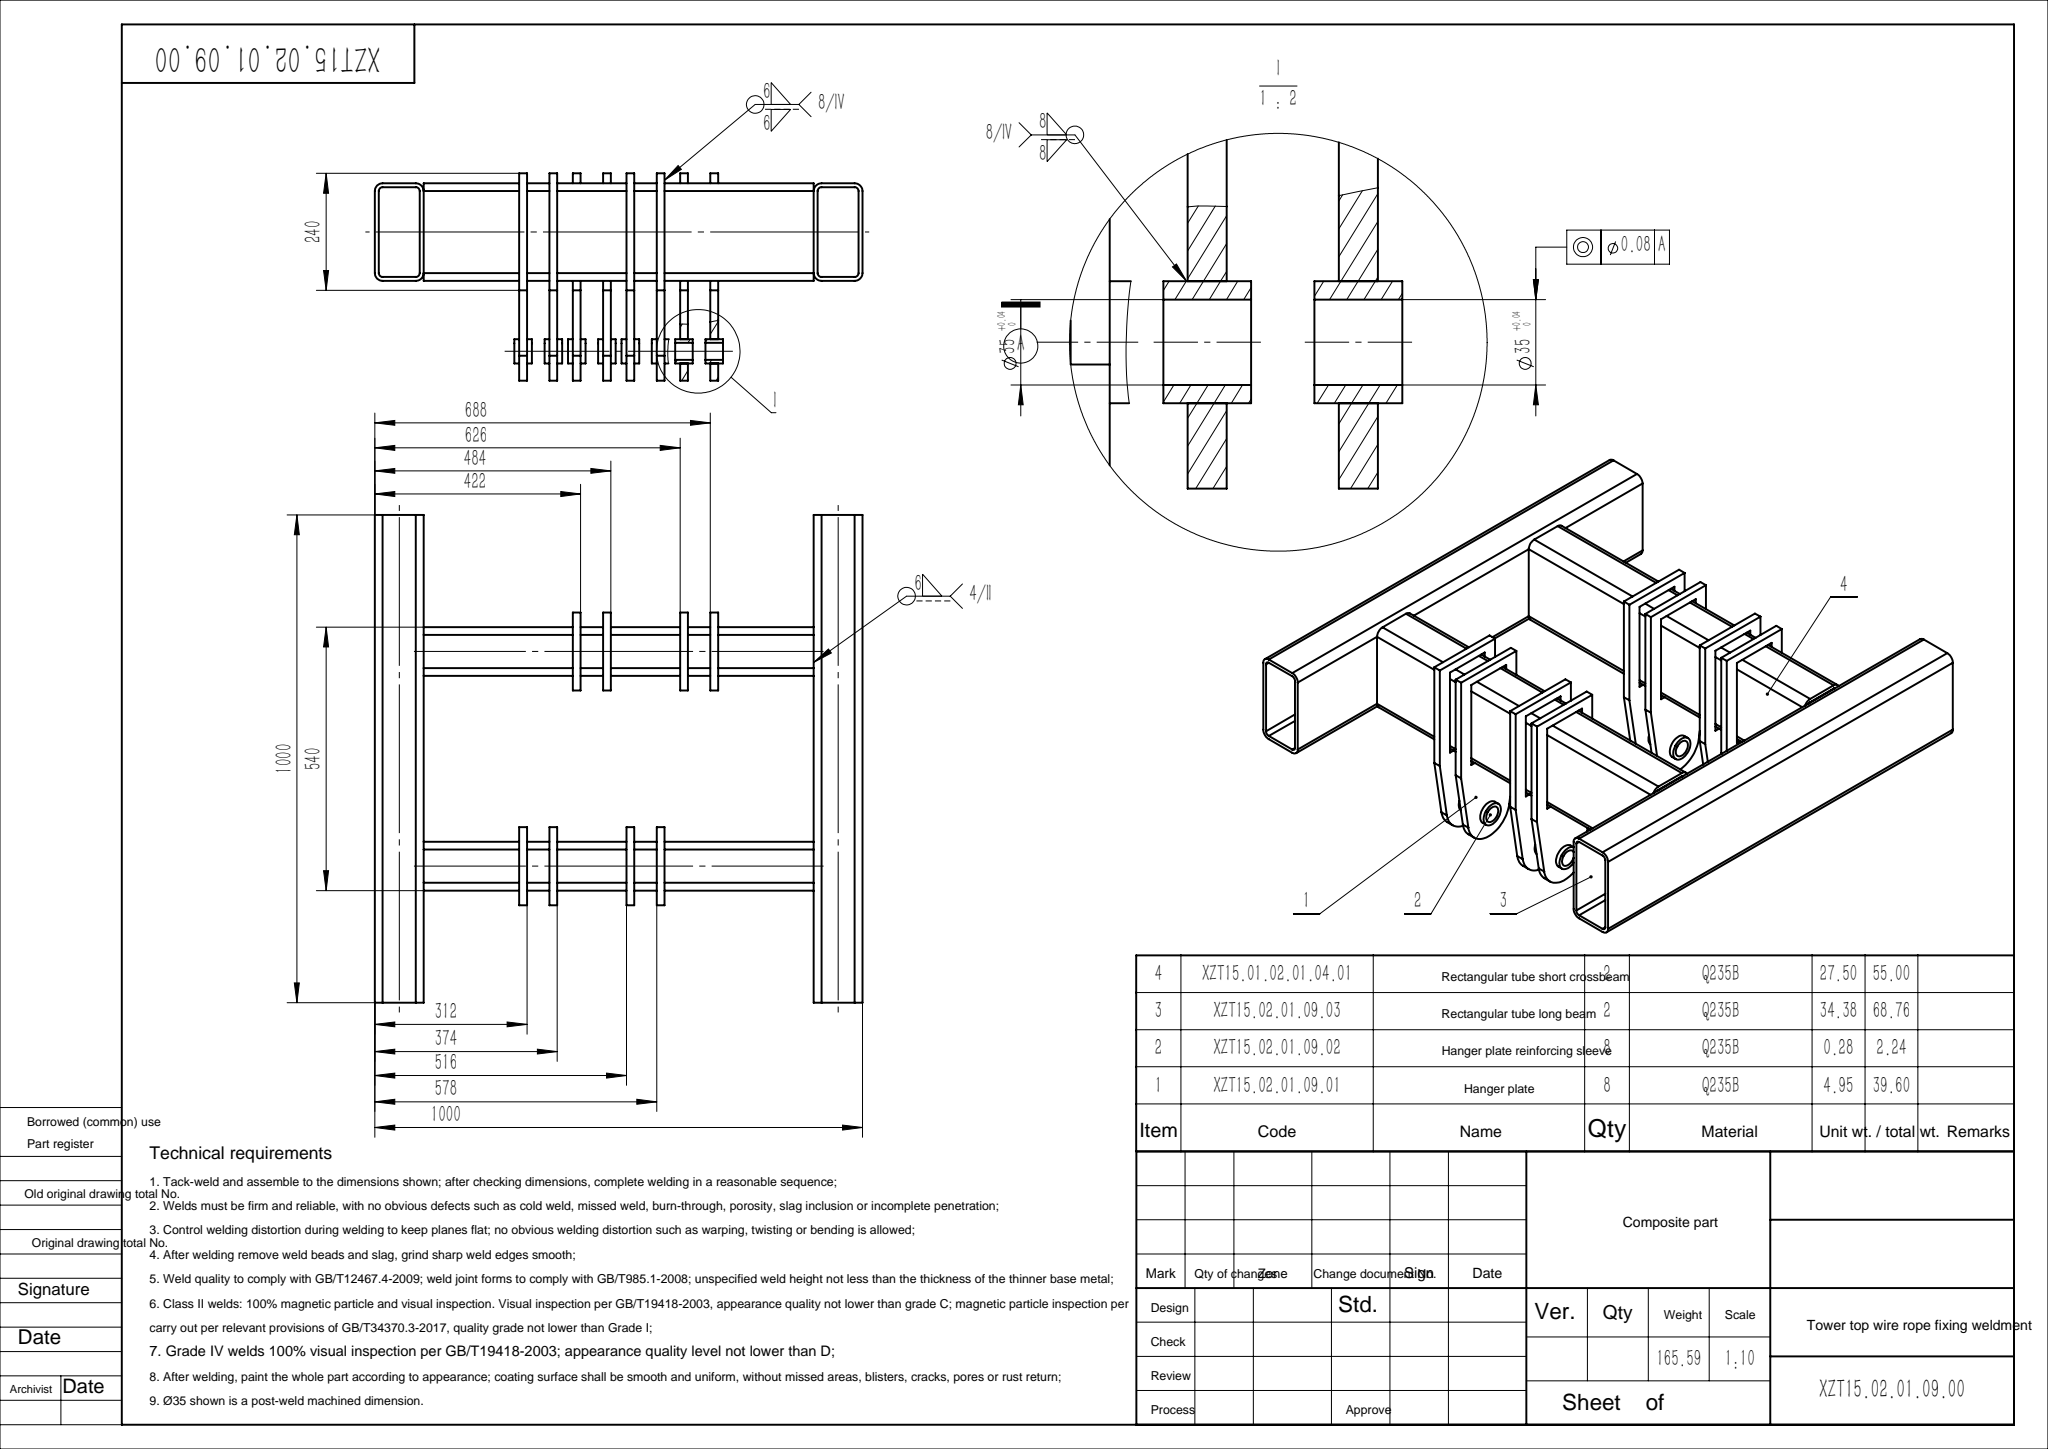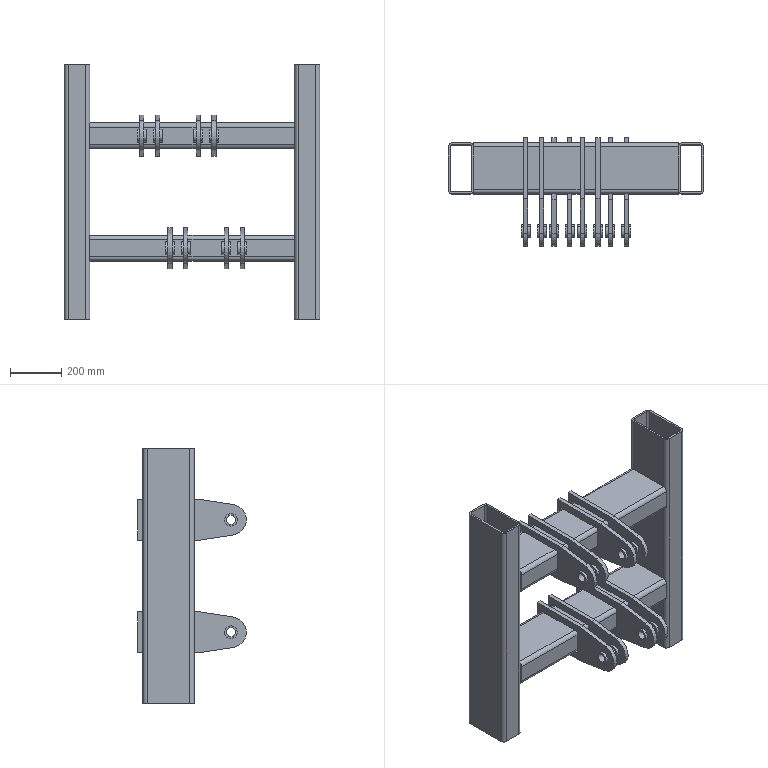Part | SolidWorks | features MirrorCompFeat 2, ReferencePattern 2 | 20 solids | 232 faces | box 1000 x 425 x 1000 mm | volume 21094555 mm3 | plane 144 | cylinder 88 | commonest cylinder face diameters 50 x32 16 x16 32 x16 35 x16 120 x8